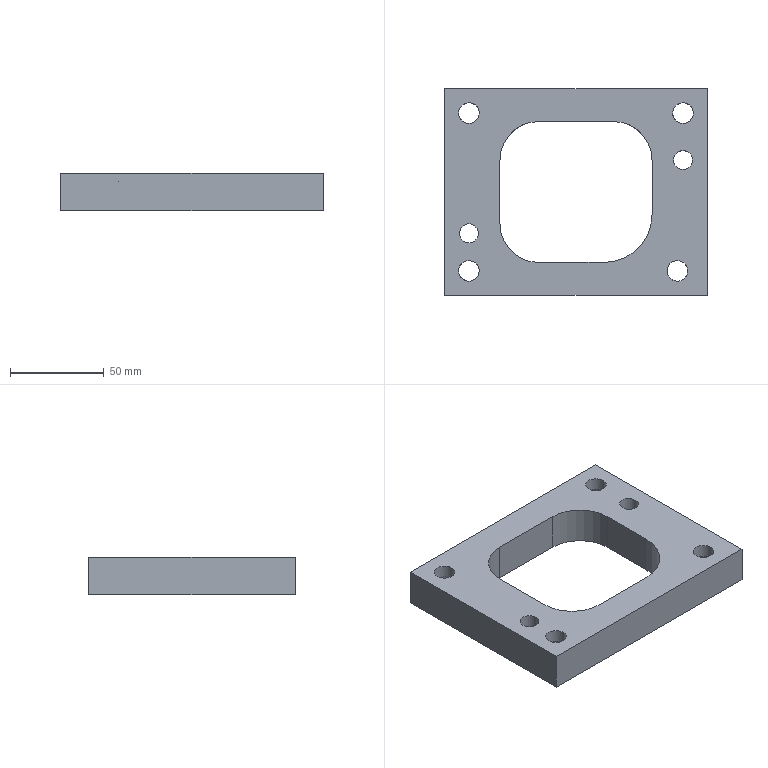Part | STEP file | 400_id2290_x_t | 1 solid | 32 faces | box 140 x 110 x 20 mm | volume 176767 mm3 | plane 16 | cylinder 16 | commonest cylinder face diameters 11 x6 17 x4 41 x3 10 x2 51 x1